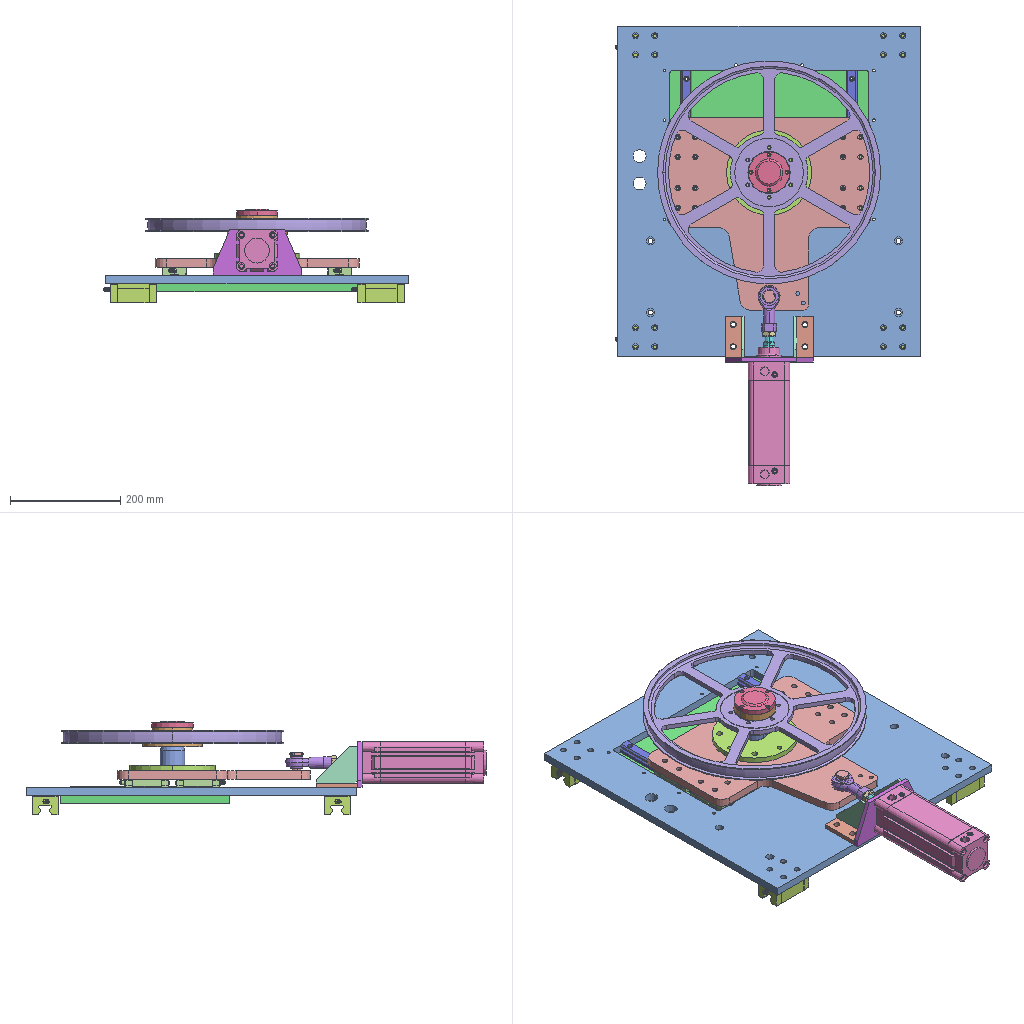Assembly | SolidWorks | 28 different items | 40 placed | box 554 x 835 x 170 mm
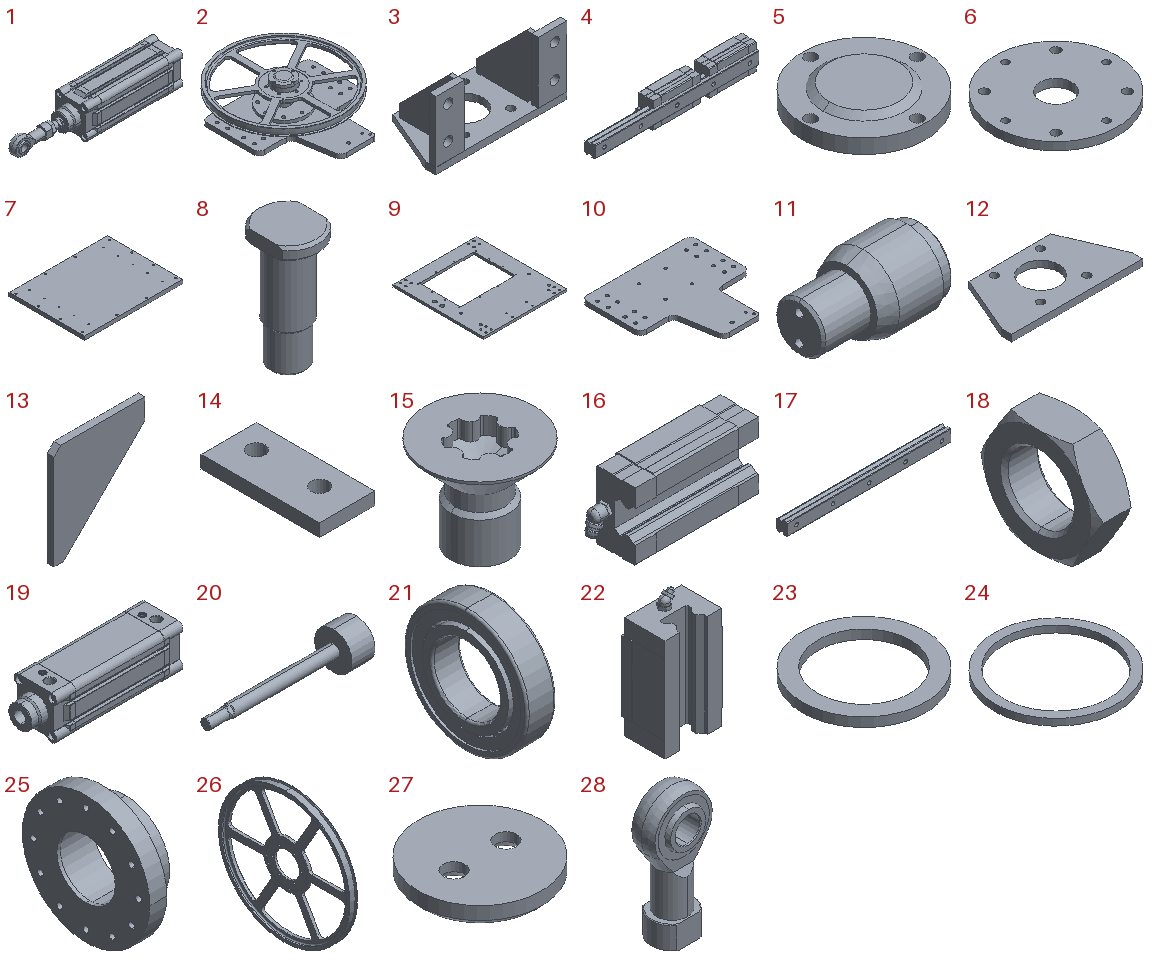Parts list (item | name | quantity | parent item | size | volume | features):
1 | (subassembly) | x1 | - | 364 x 75 x 75 mm | 905739 mm3 | -
2 | (subassembly) | x1 | - | 405 x 452.5 x 105 mm | 2366410 mm3 | -
3 | (subassembly) | x1 | - | 160 x 82.5 x 83 mm | 145011 mm3 | -
4 | (subassembly) | x2 | - | 281.473 x 30 x 44 mm | 214734 mm3 | -
5 | - | x1 | in 2 | 75 x 75 x 13.8 mm | 30557 mm3 | features BaseBody 1, Chamfer 1
6 | - | x1 | in 2 | 155 x 155 x 10 mm | 169991 mm3 | features BaseBody 1, ICE 1
7 | - | x1 | - | 400 x 308 x 15 mm | 1834801 mm3 | features BaseBody 1
8 | - | x1 | - | 19 x 24 x 48 mm | 9861 mm3 | features BaseBody 1
9 | - | x1 | - | 550 x 600 x 15 mm | 3438854 mm3 | features BaseBody 1, ICE 1
10 | - | x1 | in 2 | 370 x 350 x 15 mm | 1392433 mm3 | features ICE 4, BaseBody 1, Fillet 1
11 | - | x1 | in 2 | 74 x 45 x 45 mm | 86191 mm3 | features BaseBody 1
12 | - | x1 | in 3 | 160 x 82.5 x 8 mm | 73927 mm3 | features BaseBody 1, ICE 1
13 | - | x2 | in 3 | 67 x 5 x 75 mm | 16062 mm3 | features BaseBody 1, Chamfer 1
14 | - | x2 | in 3 | 35 x 75 x 8 mm | 19479 mm3 | features BaseBody 1
15 | - | x2 | in 2 | 11.3 x 11.3 x 10 mm | 323.209 mm3 | features BaseBody 1
16 | - | x4 | in 4 | 90.473 x 25.7 x 44 mm | 66840 mm3 | features BaseBody 1
17 | - | x2 | in 4 | 270 x 17.5 x 20 mm | 81053 mm3 | features BaseBody 1
18 | - | x1 | in 1 | 8 x 26.558 x 23 mm | 2309 mm3 | features BaseBody 1
19 | - | x1 | in 1 | 252 x 75 x 75 mm | 699508 mm3 | features BaseBody 1
20 | - | x1 | in 1 | 248.5 x 61.5 x 61.5 mm | 175012 mm3 | features BaseBody 1
21 | - | x2 | in 2 | 13 x 55 x 55 mm | 14054 mm3 | features BaseBody 1
22 | - | x4 | - | 48 x 34.5 x 96 mm | 106215 mm3 | features BaseBody 1
23 | - | x1 | in 2 | 40 x 40 x 3 mm | 1649 mm3 | features BaseBody 1
24 | - | x1 | in 2 | 55 x 55 x 3 mm | 1923 mm3 | features BaseBody 1
25 | - | x1 | in 2 | 34 x 109 x 109 mm | 138553 mm3 | features BaseBody 1, CirPattern 1, HoleWzd 1, ICE 1
26 | - | x1 | in 2 | 25 x 405 x 405 mm | 510494 mm3 | features BaseBody 1
27 | - | x1 | in 2 | 38 x 38 x 6 mm | 5863 mm3 | features BaseBody 1
28 | - | x1 | in 1 | 40 x 22 x 84 mm | 28909 mm3 | features MBimport 1
Mates (type | each side: item.copy, entity, surface, feature):
Concentric | 20.1 face cylinder Imported1 | 28.1 face cylinder F-M16X150U.stp
Coincident | 18.1 face plane Imported1 | 28.1 face plane F-M16X150U.stp
Parallel | 19.1 face plane Imported1 | 28.1 face plane F-M16X150U.stp
DistanceDim | 18.1 face | 20.1 face plane Imported1